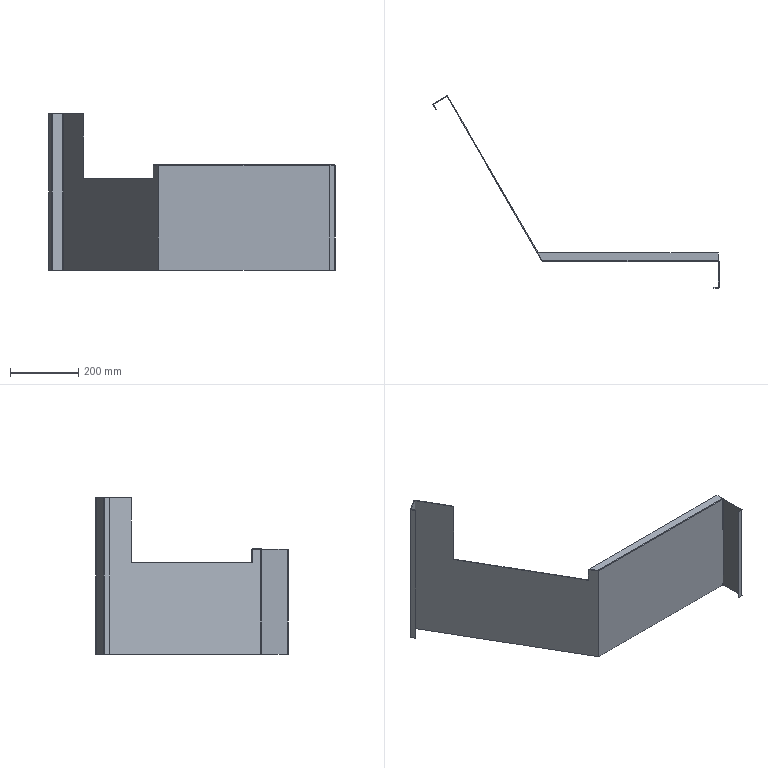Part | STEP file | zh001 | 1 solid | 42 faces | box 840.386 x 564.059 x 459.75 mm | volume 808463 mm3 | plane 28 | cylinder 14 | commonest cylinder face diameters 1 x7 5 x7
STEP:
#1=CARTESIAN_POINT('',(-569.929,497.059,459.75));
#2=VERTEX_POINT('',#1);
#3=CARTESIAN_POINT('',(-569.595,495.809,459.75));
#4=VERTEX_POINT('',#3);
#5=CARTESIAN_POINT('',(-567.429,497.059,459.75));
#6=DIRECTION('',(0.,0.,1.));
#7=DIRECTION('',(-1.,0.,0.));
#8=AXIS2_PLACEMENT_3D('',#5,#6,#7);
#9=CIRCLE('',#8,2.5);
#10=EDGE_CURVE('',#2,#4,#9,.T.);
#11=ORIENTED_EDGE('',*,*,#10,.F.);
#12=CARTESIAN_POINT('',(-569.929,497.059,0.));
#13=VERTEX_POINT('',#12);
#14=CARTESIAN_POINT('',(-569.929,497.059,308.));
#15=DIRECTION('',(0.,0.,-1.));
#16=VECTOR('',#15,1000.);
#17=LINE('',#14,#16);
#18=EDGE_CURVE('',#2,#13,#17,.T.);
#19=ORIENTED_EDGE('',*,*,#18,.T.);
#20=CARTESIAN_POINT('',(-569.595,495.809,0.));
#21=VERTEX_POINT('',#20);
#22=CARTESIAN_POINT('',(-567.429,497.059,0.));
#23=DIRECTION('',(0.,0.,1.));
#24=DIRECTION('',(-1.,0.,0.));
#25=AXIS2_PLACEMENT_3D('',#22,#23,#24);
#26=CIRCLE('',#25,2.5);
#27=EDGE_CURVE('',#13,#21,#26,.T.);
#28=ORIENTED_EDGE('',*,*,#27,.T.);
#29=CARTESIAN_POINT('',(-569.595,495.809,308.));
#30=DIRECTION('',(0.,0.,1.));
#31=VECTOR('',#30,1000.);
#32=LINE('',#29,#31);
#33=EDGE_CURVE('',#21,#4,#32,.T.);
#34=ORIENTED_EDGE('',*,*,#33,.T.);
#35=EDGE_LOOP('',(#11,#19,#28,#34));
#36=FACE_OUTER_BOUND('',#35,.T.);
#37=CARTESIAN_POINT('',(-567.429,497.059,308.));
#38=DIRECTION('',(0.,0.,-1.));
#39=DIRECTION('',(-1.,0.,0.));
#40=AXIS2_PLACEMENT_3D('',#37,#38,#39);
#41=CYLINDRICAL_SURFACE('',#40,2.5);
#42=ADVANCED_FACE('',(#36),#41,.T.);
#43=CARTESIAN_POINT('',(-567.929,497.059,459.75));
#44=VERTEX_POINT('',#43);
#45=CARTESIAN_POINT('',(-567.679,497.492,459.75));
#46=VERTEX_POINT('',#45);
#47=CARTESIAN_POINT('',(-567.429,497.059,459.75));
#48=DIRECTION('',(0.,0.,-1.));
#49=DIRECTION('',(-1.,0.,0.));
#50=AXIS2_PLACEMENT_3D('',#47,#48,#49);
#51=CIRCLE('',#50,0.5);
#52=EDGE_CURVE('',#44,#46,#51,.T.);
#53=ORIENTED_EDGE('',*,*,#52,.F.);
#54=CARTESIAN_POINT('',(-567.929,497.059,0.));
#55=VERTEX_POINT('',#54);
#56=CARTESIAN_POINT('',(-567.929,497.059,308.));
#57=DIRECTION('',(0.,0.,-1.));
#58=VECTOR('',#57,1000.);
#59=LINE('',#56,#58);
#60=EDGE_CURVE('',#44,#55,#59,.T.);
#61=ORIENTED_EDGE('',*,*,#60,.T.);
#62=CARTESIAN_POINT('',(-567.679,497.492,0.));
#63=VERTEX_POINT('',#62);
#64=CARTESIAN_POINT('',(-567.429,497.059,0.));
#65=DIRECTION('',(0.,0.,1.));
#66=DIRECTION('',(-1.,0.,0.));
#67=AXIS2_PLACEMENT_3D('',#64,#65,#66);
#68=CIRCLE('',#67,0.5);
#69=EDGE_CURVE('',#63,#55,#68,.T.);
#70=ORIENTED_EDGE('',*,*,#69,.F.);
#71=CARTESIAN_POINT('',(-567.679,497.492,308.));
#72=DIRECTION('',(0.,0.,-1.));
#73=VECTOR('',#72,1000.);
#74=LINE('',#71,#73);
#75=EDGE_CURVE('',#46,#63,#74,.T.);
#76=ORIENTED_EDGE('',*,*,#75,.F.);
#77=EDGE_LOOP('',(#53,#61,#70,#76));
#78=FACE_OUTER_BOUND('',#77,.T.);
#79=CARTESIAN_POINT('',(-567.429,497.059,308.));
#80=DIRECTION('',(0.,0.,-1.));
#81=DIRECTION('',(-1.,0.,0.));
#82=AXIS2_PLACEMENT_3D('',#79,#80,#81);
#83=CYLINDRICAL_SURFACE('',#82,0.5);
#84=ADVANCED_FACE('',(#78),#83,.F.);
#85=CARTESIAN_POINT('',(-467.543,419.051,459.75));
#86=VERTEX_POINT('',#85);
#87=CARTESIAN_POINT('',(-526.293,520.809,459.75));
#88=VERTEX_POINT('',#87);
#89=CARTESIAN_POINT('',(-247.543,38.,459.75));
#90=DIRECTION('',(-0.5,0.866,0.));
#91=VECTOR('',#90,1000.);
#92=LINE('',#89,#91);
#93=EDGE_CURVE('',#86,#88,#92,.T.);
#94=ORIENTED_EDGE('',*,*,#93,.F.);
#95=CARTESIAN_POINT('',(-467.543,419.051,269.5));
#96=VERTEX_POINT('',#95);
#97=CARTESIAN_POINT('',(-467.543,419.051,308.));
#98=DIRECTION('',(0.,0.,1.));
#99=VECTOR('',#98,1000.);
#100=LINE('',#97,#99);
#101=EDGE_CURVE('',#96,#86,#100,.T.);
#102=ORIENTED_EDGE('',*,*,#101,.F.);
#103=CARTESIAN_POINT('',(-262.471,63.856,269.5));
#104=VERTEX_POINT('',#103);
#105=CARTESIAN_POINT('',(-247.543,38.,269.5));
#106=DIRECTION('',(-0.5,0.866,0.));
#107=VECTOR('',#106,1000.);
#108=LINE('',#105,#107);
#109=EDGE_CURVE('',#104,#96,#108,.T.);
#110=ORIENTED_EDGE('',*,*,#109,.F.);
#111=CARTESIAN_POINT('',(-262.471,63.856,308.));
#112=VERTEX_POINT('',#111);
#113=CARTESIAN_POINT('',(-262.471,63.856,308.));
#114=DIRECTION('',(0.,0.,-1.));
#115=VECTOR('',#114,1000.);
#116=LINE('',#113,#115);
#117=EDGE_CURVE('',#112,#104,#116,.T.);
#118=ORIENTED_EDGE('',*,*,#117,.F.);
#119=CARTESIAN_POINT('',(-247.688,38.25,308.));
#120=VERTEX_POINT('',#119);
#121=CARTESIAN_POINT('',(-247.543,38.,308.));
#122=DIRECTION('',(-0.5,0.866,0.));
#123=VECTOR('',#122,1000.);
#124=LINE('',#121,#123);
#125=EDGE_CURVE('',#120,#112,#124,.T.);
#126=ORIENTED_EDGE('',*,*,#125,.F.);
#127=CARTESIAN_POINT('',(-247.688,38.25,0.));
#128=VERTEX_POINT('',#127);
#129=CARTESIAN_POINT('',(-247.688,38.25,308.));
#130=DIRECTION('',(0.,0.,1.));
#131=VECTOR('',#130,1000.);
#132=LINE('',#129,#131);
#133=EDGE_CURVE('',#128,#120,#132,.T.);
#134=ORIENTED_EDGE('',*,*,#133,.F.);
#135=CARTESIAN_POINT('',(-526.293,520.809,0.));
#136=VERTEX_POINT('',#135);
#137=CARTESIAN_POINT('',(-247.543,38.,0.));
#138=DIRECTION('',(0.5,-0.866,0.));
#139=VECTOR('',#138,1000.);
#140=LINE('',#137,#139);
#141=EDGE_CURVE('',#136,#128,#140,.T.);
#142=ORIENTED_EDGE('',*,*,#141,.F.);
#143=CARTESIAN_POINT('',(-526.293,520.809,308.));
#144=DIRECTION('',(0.,0.,-1.));
#145=VECTOR('',#144,1000.);
#146=LINE('',#143,#145);
#147=EDGE_CURVE('',#88,#136,#146,.T.);
#148=ORIENTED_EDGE('',*,*,#147,.F.);
#149=EDGE_LOOP('',(#94,#102,#110,#118,#126,#134,#142,#148));
#150=FACE_OUTER_BOUND('',#149,.T.);
#151=CARTESIAN_POINT('',(-247.543,38.,308.));
#152=DIRECTION('',(-0.866,-0.5,0.));
#153=DIRECTION('',(0.5,-0.866,0.));
#154=AXIS2_PLACEMENT_3D('',#151,#152,#153);
#155=PLANE('',#154);
#156=ADVANCED_FACE('',(#150),#155,.F.);
#157=CARTESIAN_POINT('',(-529.708,521.724,459.75));
#158=VERTEX_POINT('',#157);
#159=CARTESIAN_POINT('',(-528.458,519.559,459.75));
#160=DIRECTION('',(0.,0.,-1.));
#161=DIRECTION('',(-1.,0.,0.));
#162=AXIS2_PLACEMENT_3D('',#159,#160,#161);
#163=CIRCLE('',#162,2.5);
#164=EDGE_CURVE('',#158,#88,#163,.T.);
#165=ORIENTED_EDGE('',*,*,#164,.T.);
#166=ORIENTED_EDGE('',*,*,#147,.T.);
#167=CARTESIAN_POINT('',(-529.708,521.724,0.));
#168=VERTEX_POINT('',#167);
#169=CARTESIAN_POINT('',(-528.458,519.559,0.));
#170=DIRECTION('',(0.,0.,1.));
#171=DIRECTION('',(-1.,0.,0.));
#172=AXIS2_PLACEMENT_3D('',#169,#170,#171);
#173=CIRCLE('',#172,2.5);
#174=EDGE_CURVE('',#136,#168,#173,.T.);
#175=ORIENTED_EDGE('',*,*,#174,.T.);
#176=CARTESIAN_POINT('',(-529.708,521.724,308.));
#177=DIRECTION('',(0.,0.,1.));
#178=VECTOR('',#177,1000.);
#179=LINE('',#176,#178);
#180=EDGE_CURVE('',#168,#158,#179,.T.);
#181=ORIENTED_EDGE('',*,*,#180,.T.);
#182=EDGE_LOOP('',(#165,#166,#175,#181));
#183=FACE_OUTER_BOUND('',#182,.T.);
#184=CARTESIAN_POINT('',(-528.458,519.559,308.));
#185=DIRECTION('',(0.,0.,-1.));
#186=DIRECTION('',(-1.,0.,0.));
#187=AXIS2_PLACEMENT_3D('',#184,#185,#186);
#188=CYLINDRICAL_SURFACE('',#187,2.5);
#189=ADVANCED_FACE('',(#183),#188,.T.);
#190=CARTESIAN_POINT('',(-528.708,519.992,459.75));
#191=VERTEX_POINT('',#190);
#192=CARTESIAN_POINT('',(-528.025,519.809,459.75));
#193=VERTEX_POINT('',#192);
#194=CARTESIAN_POINT('',(-528.458,519.559,459.75));
#195=DIRECTION('',(0.,0.,-1.));
#196=DIRECTION('',(-1.,0.,0.));
#197=AXIS2_PLACEMENT_3D('',#194,#195,#196);
#198=CIRCLE('',#197,0.5);
#199=EDGE_CURVE('',#191,#193,#198,.T.);
#200=ORIENTED_EDGE('',*,*,#199,.T.);
#201=CARTESIAN_POINT('',(-469.275,418.051,459.75));
#202=VERTEX_POINT('',#201);
#203=CARTESIAN_POINT('',(-528.025,519.809,459.75));
#204=DIRECTION('',(0.5,-0.866,0.));
#205=VECTOR('',#204,1000.);
#206=LINE('',#203,#205);
#207=EDGE_CURVE('',#193,#202,#206,.T.);
#208=ORIENTED_EDGE('',*,*,#207,.T.);
#209=CARTESIAN_POINT('',(-469.275,418.051,459.75));
#210=DIRECTION('',(0.866,0.5,0.));
#211=VECTOR('',#210,1000.);
#212=LINE('',#209,#211);
#213=EDGE_CURVE('',#202,#86,#212,.T.);
#214=ORIENTED_EDGE('',*,*,#213,.T.);
#215=ORIENTED_EDGE('',*,*,#93,.T.);
#216=ORIENTED_EDGE('',*,*,#164,.F.);
#217=CARTESIAN_POINT('',(-568.679,499.224,459.75));
#218=VERTEX_POINT('',#217);
#219=CARTESIAN_POINT('',(-529.708,521.724,459.75));
#220=DIRECTION('',(-0.866,-0.5,0.));
#221=VECTOR('',#220,1000.);
#222=LINE('',#219,#221);
#223=EDGE_CURVE('',#158,#218,#222,.T.);
#224=ORIENTED_EDGE('',*,*,#223,.T.);
#225=CARTESIAN_POINT('',(-567.429,497.059,459.75));
#226=DIRECTION('',(0.,0.,1.));
#227=DIRECTION('',(-1.,0.,0.));
#228=AXIS2_PLACEMENT_3D('',#225,#226,#227);
#229=CIRCLE('',#228,2.5);
#230=EDGE_CURVE('',#218,#2,#229,.T.);
#231=ORIENTED_EDGE('',*,*,#230,.T.);
#232=ORIENTED_EDGE('',*,*,#10,.T.);
#233=CARTESIAN_POINT('',(-561.845,482.386,459.75));
#234=VERTEX_POINT('',#233);
#235=CARTESIAN_POINT('',(-569.595,495.809,459.75));
#236=DIRECTION('',(0.5,-0.866,0.));
#237=VECTOR('',#236,1000.);
#238=LINE('',#235,#237);
#239=EDGE_CURVE('',#4,#234,#238,.T.);
#240=ORIENTED_EDGE('',*,*,#239,.T.);
#241=CARTESIAN_POINT('',(-560.113,483.386,459.75));
#242=VERTEX_POINT('',#241);
#243=CARTESIAN_POINT('',(-561.845,482.386,459.75));
#244=DIRECTION('',(0.866,0.5,0.));
#245=VECTOR('',#244,1000.);
#246=LINE('',#243,#245);
#247=EDGE_CURVE('',#234,#242,#246,.T.);
#248=ORIENTED_EDGE('',*,*,#247,.T.);
#249=CARTESIAN_POINT('',(-567.863,496.809,459.75));
#250=VERTEX_POINT('',#249);
#251=CARTESIAN_POINT('',(-560.113,483.386,459.75));
#252=DIRECTION('',(-0.5,0.866,0.));
#253=VECTOR('',#252,1000.);
#254=LINE('',#251,#253);
#255=EDGE_CURVE('',#242,#250,#254,.T.);
#256=ORIENTED_EDGE('',*,*,#255,.T.);
#257=CARTESIAN_POINT('',(-567.429,497.059,459.75));
#258=DIRECTION('',(0.,0.,-1.));
#259=DIRECTION('',(-1.,0.,0.));
#260=AXIS2_PLACEMENT_3D('',#257,#258,#259);
#261=CIRCLE('',#260,0.5);
#262=EDGE_CURVE('',#250,#44,#261,.T.);
#263=ORIENTED_EDGE('',*,*,#262,.T.);
#264=ORIENTED_EDGE('',*,*,#52,.T.);
#265=CARTESIAN_POINT('',(-567.679,497.492,459.75));
#266=DIRECTION('',(0.866,0.5,0.));
#267=VECTOR('',#266,1000.);
#268=LINE('',#265,#267);
#269=EDGE_CURVE('',#46,#191,#268,.T.);
#270=ORIENTED_EDGE('',*,*,#269,.T.);
#271=EDGE_LOOP('',(#200,#208,#214,#215,#216,#224,#231,#232,#240,#248,#256,#263,#264,#270));
#272=FACE_OUTER_BOUND('',#271,.T.);
#273=CARTESIAN_POINT('',(-528.458,519.559,459.75));
#274=DIRECTION('',(0.,0.,1.));
#275=DIRECTION('',(1.,0.,0.));
#276=AXIS2_PLACEMENT_3D('',#273,#274,#275);
#277=PLANE('',#276);
#278=ADVANCED_FACE('',(#272),#277,.T.);
#279=ORIENTED_EDGE('',*,*,#213,.F.);
#280=CARTESIAN_POINT('',(-469.275,418.051,269.5));
#281=VERTEX_POINT('',#280);
#282=CARTESIAN_POINT('',(-469.275,418.051,308.));
#283=DIRECTION('',(0.,0.,1.));
#284=VECTOR('',#283,1000.);
#285=LINE('',#282,#284);
#286=EDGE_CURVE('',#281,#202,#285,.T.);
#287=ORIENTED_EDGE('',*,*,#286,.F.);
#288=CARTESIAN_POINT('',(-469.275,418.051,269.5));
#289=DIRECTION('',(-0.866,-0.5,0.));
#290=VECTOR('',#289,1000.);
#291=LINE('',#288,#290);
#292=EDGE_CURVE('',#96,#281,#291,.T.);
#293=ORIENTED_EDGE('',*,*,#292,.F.);
#294=ORIENTED_EDGE('',*,*,#101,.T.);
#295=EDGE_LOOP('',(#279,#287,#293,#294));
#296=FACE_OUTER_BOUND('',#295,.T.);
#297=CARTESIAN_POINT('',(-469.275,418.051,308.));
#298=DIRECTION('',(-0.5,0.866,0.));
#299=DIRECTION('',(-0.866,-0.5,0.));
#300=AXIS2_PLACEMENT_3D('',#297,#298,#299);
#301=PLANE('',#300);
#302=ADVANCED_FACE('',(#296),#301,.F.);
#303=ORIENTED_EDGE('',*,*,#292,.T.);
#304=CARTESIAN_POINT('',(-264.203,62.856,269.5));
#305=VERTEX_POINT('',#304);
#306=CARTESIAN_POINT('',(-264.203,62.856,269.5));
#307=DIRECTION('',(-0.5,0.866,0.));
#308=VECTOR('',#307,1000.);
#309=LINE('',#306,#308);
#310=EDGE_CURVE('',#305,#281,#309,.T.);
#311=ORIENTED_EDGE('',*,*,#310,.F.);
#312=CARTESIAN_POINT('',(-262.471,63.856,269.5));
#313=DIRECTION('',(-0.866,-0.5,0.));
#314=VECTOR('',#313,1000.);
#315=LINE('',#312,#314);
#316=EDGE_CURVE('',#104,#305,#315,.T.);
#317=ORIENTED_EDGE('',*,*,#316,.F.);
#318=ORIENTED_EDGE('',*,*,#109,.T.);
#319=EDGE_LOOP('',(#303,#311,#317,#318));
#320=FACE_OUTER_BOUND('',#319,.T.);
#321=CARTESIAN_POINT('',(-469.275,418.051,269.5));
#322=DIRECTION('',(0.,0.,-1.));
#323=DIRECTION('',(0.,1.,0.));
#324=AXIS2_PLACEMENT_3D('',#321,#322,#323);
#325=PLANE('',#324);
#326=ADVANCED_FACE('',(#320),#325,.F.);
#327=ORIENTED_EDGE('',*,*,#316,.T.);
#328=CARTESIAN_POINT('',(-264.203,62.856,308.));
#329=VERTEX_POINT('',#328);
#330=CARTESIAN_POINT('',(-264.203,62.856,308.));
#331=DIRECTION('',(0.,0.,-1.));
#332=VECTOR('',#331,1000.);
#333=LINE('',#330,#332);
#334=EDGE_CURVE('',#329,#305,#333,.T.);
#335=ORIENTED_EDGE('',*,*,#334,.F.);
#336=CARTESIAN_POINT('',(-264.203,62.856,308.));
#337=DIRECTION('',(-0.866,-0.5,0.));
#338=VECTOR('',#337,1000.);
#339=LINE('',#336,#338);
#340=EDGE_CURVE('',#112,#329,#339,.T.);
#341=ORIENTED_EDGE('',*,*,#340,.F.);
#342=ORIENTED_EDGE('',*,*,#117,.T.);
#343=EDGE_LOOP('',(#327,#335,#341,#342));
#344=FACE_OUTER_BOUND('',#343,.T.);
#345=CARTESIAN_POINT('',(-264.203,62.856,308.));
#346=DIRECTION('',(0.5,-0.866,0.));
#347=DIRECTION('',(0.866,0.5,0.));
#348=AXIS2_PLACEMENT_3D('',#345,#346,#347);
#349=PLANE('',#348);
#350=ADVANCED_FACE('',(#344),#349,.F.);
#351=CARTESIAN_POINT('',(-249.42,37.25,308.));
#352=VERTEX_POINT('',#351);
#353=CARTESIAN_POINT('',(-264.203,62.856,308.));
#354=DIRECTION('',(0.5,-0.866,0.));
#355=VECTOR('',#354,1000.);
#356=LINE('',#353,#355);
#357=EDGE_CURVE('',#329,#352,#356,.T.);
#358=ORIENTED_EDGE('',*,*,#357,.T.);
#359=CARTESIAN_POINT('',(-247.255,36.,308.));
#360=VERTEX_POINT('',#359);
#361=CARTESIAN_POINT('',(-247.255,38.5,308.));
#362=DIRECTION('',(0.,0.,1.));
#363=DIRECTION('',(-1.,0.,0.));
#364=AXIS2_PLACEMENT_3D('',#361,#362,#363);
#365=CIRCLE('',#364,2.5);
#366=EDGE_CURVE('',#352,#360,#365,.T.);
#367=ORIENTED_EDGE('',*,*,#366,.T.);
#368=CARTESIAN_POINT('',(-247.255,38.,308.));
#369=VERTEX_POINT('',#368);
#370=CARTESIAN_POINT('',(-247.255,38.,308.));
#371=DIRECTION('',(0.,1.,0.));
#372=VECTOR('',#371,1000.);
#373=LINE('',#370,#372);
#374=EDGE_CURVE('',#360,#369,#373,.T.);
#375=ORIENTED_EDGE('',*,*,#374,.T.);
#376=CARTESIAN_POINT('',(-247.255,38.5,308.));
#377=DIRECTION('',(0.,0.,-1.));
#378=DIRECTION('',(-1.,0.,0.));
#379=AXIS2_PLACEMENT_3D('',#376,#377,#378);
#380=CIRCLE('',#379,0.5);
#381=EDGE_CURVE('',#369,#120,#380,.T.);
#382=ORIENTED_EDGE('',*,*,#381,.T.);
#383=ORIENTED_EDGE('',*,*,#125,.T.);
#384=ORIENTED_EDGE('',*,*,#340,.T.);
#385=EDGE_LOOP('',(#358,#367,#375,#382,#383,#384));
#386=FACE_OUTER_BOUND('',#385,.T.);
#387=CARTESIAN_POINT('',(-528.708,519.992,308.));
#388=DIRECTION('',(0.,0.,1.));
#389=DIRECTION('',(1.,0.,0.));
#390=AXIS2_PLACEMENT_3D('',#387,#388,#389);
#391=PLANE('',#390);
#392=ADVANCED_FACE('',(#386),#391,.T.);
#393=ORIENTED_EDGE('',*,*,#133,.T.);
#394=ORIENTED_EDGE('',*,*,#381,.F.);
#395=CARTESIAN_POINT('',(-247.255,38.,0.));
#396=VERTEX_POINT('',#395);
#397=CARTESIAN_POINT('',(-247.255,38.,308.));
#398=DIRECTION('',(0.,0.,1.));
#399=VECTOR('',#398,1000.);
#400=LINE('',#397,#399);
#401=EDGE_CURVE('',#396,#369,#400,.T.);
#402=ORIENTED_EDGE('',*,*,#401,.F.);
#403=CARTESIAN_POINT('',(-247.255,38.5,0.));
#404=DIRECTION('',(0.,0.,1.));
#405=DIRECTION('',(-1.,0.,0.));
#406=AXIS2_PLACEMENT_3D('',#403,#404,#405);
#407=CIRCLE('',#406,0.5);
#408=EDGE_CURVE('',#128,#396,#407,.T.);
#409=ORIENTED_EDGE('',*,*,#408,.F.);
#410=EDGE_LOOP('',(#393,#394,#402,#409));
#411=FACE_OUTER_BOUND('',#410,.T.);
#412=CARTESIAN_POINT('',(-247.255,38.5,308.));
#413=DIRECTION('',(0.,0.,-1.));
#414=DIRECTION('',(-1.,0.,0.));
#415=AXIS2_PLACEMENT_3D('',#412,#413,#414);
#416=CYLINDRICAL_SURFACE('',#415,0.5);
#417=ADVANCED_FACE('',(#411),#416,.F.);
#418=CARTESIAN_POINT('',(-249.42,37.25,0.));
#419=VERTEX_POINT('',#418);
#420=CARTESIAN_POINT('',(-528.025,519.809,0.));
#421=VERTEX_POINT('',#420);
#422=CARTESIAN_POINT('',(-249.42,37.25,0.));
#423=DIRECTION('',(-0.5,0.866,0.));
#424=VECTOR('',#423,1000.);
#425=LINE('',#422,#424);
#426=EDGE_CURVE('',#419,#421,#425,.T.);
#427=ORIENTED_EDGE('',*,*,#426,.T.);
#428=CARTESIAN_POINT('',(-528.708,519.992,0.));
#429=VERTEX_POINT('',#428);
#430=CARTESIAN_POINT('',(-528.458,519.559,0.));
#431=DIRECTION('',(0.,0.,1.));
#432=DIRECTION('',(-1.,0.,0.));
#433=AXIS2_PLACEMENT_3D('',#430,#431,#432);
#434=CIRCLE('',#433,0.5);
#435=EDGE_CURVE('',#421,#429,#434,.T.);
#436=ORIENTED_EDGE('',*,*,#435,.T.);
#437=CARTESIAN_POINT('',(-526.543,521.242,0.));
#438=DIRECTION('',(0.866,0.5,0.));
#439=VECTOR('',#438,1000.);
#440=LINE('',#437,#439);
#441=EDGE_CURVE('',#63,#429,#440,.T.);
#442=ORIENTED_EDGE('',*,*,#441,.F.);
#443=ORIENTED_EDGE('',*,*,#69,.T.);
#444=CARTESIAN_POINT('',(-567.863,496.809,0.));
#445=VERTEX_POINT('',#444);
#446=CARTESIAN_POINT('',(-567.429,497.059,0.));
#447=DIRECTION('',(0.,0.,1.));
#448=DIRECTION('',(-1.,0.,0.));
#449=AXIS2_PLACEMENT_3D('',#446,#447,#448);
#450=CIRCLE('',#449,0.5);
#451=EDGE_CURVE('',#55,#445,#450,.T.);
#452=ORIENTED_EDGE('',*,*,#451,.T.);
#453=CARTESIAN_POINT('',(-560.113,483.386,0.));
#454=VERTEX_POINT('',#453);
#455=CARTESIAN_POINT('',(-569.113,498.974,0.));
#456=DIRECTION('',(-0.5,0.866,0.));
#457=VECTOR('',#456,1000.);
#458=LINE('',#455,#457);
#459=EDGE_CURVE('',#454,#445,#458,.T.);
#460=ORIENTED_EDGE('',*,*,#459,.F.);
#461=CARTESIAN_POINT('',(-561.845,482.386,0.));
#462=VERTEX_POINT('',#461);
#463=CARTESIAN_POINT('',(-560.113,483.386,0.));
#464=DIRECTION('',(0.866,0.5,0.));
#465=VECTOR('',#464,1000.);
#466=LINE('',#463,#465);
#467=EDGE_CURVE('',#462,#454,#466,.T.);
#468=ORIENTED_EDGE('',*,*,#467,.F.);
#469=CARTESIAN_POINT('',(-570.845,497.974,0.));
#470=DIRECTION('',(-0.5,0.866,0.));
#471=VECTOR('',#470,1000.);
#472=LINE('',#469,#471);
#473=EDGE_CURVE('',#462,#21,#472,.T.);
#474=ORIENTED_EDGE('',*,*,#473,.T.);
#475=ORIENTED_EDGE('',*,*,#27,.F.);
#476=CARTESIAN_POINT('',(-568.679,499.224,0.));
#477=VERTEX_POINT('',#476);
#478=CARTESIAN_POINT('',(-567.429,497.059,0.));
#479=DIRECTION('',(0.,0.,1.));
#480=DIRECTION('',(-1.,0.,0.));
#481=AXIS2_PLACEMENT_3D('',#478,#479,#480);
#482=CIRCLE('',#481,2.5);
#483=EDGE_CURVE('',#477,#13,#482,.T.);
#484=ORIENTED_EDGE('',*,*,#483,.F.);
#485=CARTESIAN_POINT('',(-527.543,522.974,0.));
#486=DIRECTION('',(0.866,0.5,0.));
#487=VECTOR('',#486,1000.);
#488=LINE('',#485,#487);
#489=EDGE_CURVE('',#477,#168,#488,.T.);
#490=ORIENTED_EDGE('',*,*,#489,.T.);
#491=ORIENTED_EDGE('',*,*,#174,.F.);
#492=ORIENTED_EDGE('',*,*,#141,.T.);
#493=ORIENTED_EDGE('',*,*,#408,.T.);
#494=CARTESIAN_POINT('',(267.957,38.,0.));
#495=VERTEX_POINT('',#494);
#496=CARTESIAN_POINT('',(270.457,38.,0.));
#497=DIRECTION('',(1.,0.,0.));
#498=VECTOR('',#497,1000.);
#499=LINE('',#496,#498);
#500=EDGE_CURVE('',#396,#495,#499,.T.);
#501=ORIENTED_EDGE('',*,*,#500,.T.);
#502=CARTESIAN_POINT('',(270.457,35.5,0.));
#503=VERTEX_POINT('',#502);
#504=CARTESIAN_POINT('',(267.957,35.5,0.));
#505=DIRECTION('',(0.,0.,1.));
#506=DIRECTION('',(-1.,0.,0.));
#507=AXIS2_PLACEMENT_3D('',#504,#505,#506);
#508=CIRCLE('',#507,2.5);
#509=EDGE_CURVE('',#503,#495,#508,.T.);
#510=ORIENTED_EDGE('',*,*,#509,.F.);
#511=CARTESIAN_POINT('',(270.457,-39.5,0.));
#512=VERTEX_POINT('',#511);
#513=CARTESIAN_POINT('',(270.457,-42.,0.));
#514=DIRECTION('',(0.,-1.,0.));
#515=VECTOR('',#514,1000.);
#516=LINE('',#513,#515);
#517=EDGE_CURVE('',#503,#512,#516,.T.);
#518=ORIENTED_EDGE('',*,*,#517,.T.);
#519=CARTESIAN_POINT('',(267.957,-42.,0.));
#520=VERTEX_POINT('',#519);
#521=CARTESIAN_POINT('',(267.957,-39.5,0.));
#522=DIRECTION('',(0.,0.,1.));
#523=DIRECTION('',(-1.,0.,0.));
#524=AXIS2_PLACEMENT_3D('',#521,#522,#523);
#525=CIRCLE('',#524,2.5);
#526=EDGE_CURVE('',#520,#512,#525,.T.);
#527=ORIENTED_EDGE('',*,*,#526,.F.);
#528=CARTESIAN_POINT('',(255.457,-42.,0.));
#529=VERTEX_POINT('',#528);
#530=CARTESIAN_POINT('',(270.457,-42.,0.));
#531=DIRECTION('',(-1.,0.,0.));
#532=VECTOR('',#531,1000.);
#533=LINE('',#530,#532);
#534=EDGE_CURVE('',#520,#529,#533,.T.);
#535=ORIENTED_EDGE('',*,*,#534,.T.);
#536=CARTESIAN_POINT('',(255.457,-40.,0.));
#537=VERTEX_POINT('',#536);
#538=CARTESIAN_POINT('',(255.457,497.059,0.));
#539=DIRECTION('',(0.,-1.,0.));
#540=VECTOR('',#539,1000.);
#541=LINE('',#538,#540);
#542=EDGE_CURVE('',#537,#529,#541,.T.);
#543=ORIENTED_EDGE('',*,*,#542,.F.);
#544=CARTESIAN_POINT('',(267.957,-40.,0.));
#545=VERTEX_POINT('',#544);
#546=CARTESIAN_POINT('',(-567.429,-40.,0.));
#547=DIRECTION('',(-1.,0.,0.));
#548=VECTOR('',#547,1000.);
#549=LINE('',#546,#548);
#550=EDGE_CURVE('',#545,#537,#549,.T.);
#551=ORIENTED_EDGE('',*,*,#550,.F.);
#552=CARTESIAN_POINT('',(268.457,-39.5,0.));
#553=VERTEX_POINT('',#552);
#554=CARTESIAN_POINT('',(267.957,-39.5,0.));
#555=DIRECTION('',(0.,0.,1.));
#556=DIRECTION('',(-1.,0.,0.));
#557=AXIS2_PLACEMENT_3D('',#554,#555,#556);
#558=CIRCLE('',#557,0.5);
#559=EDGE_CURVE('',#545,#553,#558,.T.);
#560=ORIENTED_EDGE('',*,*,#559,.T.);
#561=CARTESIAN_POINT('',(268.457,35.5,0.));
#562=VERTEX_POINT('',#561);
#563=CARTESIAN_POINT('',(268.457,-40.,0.));
#564=DIRECTION('',(0.,1.,0.));
#565=VECTOR('',#564,1000.);
#566=LINE('',#563,#565);
#567=EDGE_CURVE('',#553,#562,#566,.T.);
#568=ORIENTED_EDGE('',*,*,#567,.T.);
#569=CARTESIAN_POINT('',(267.957,36.,0.));
#570=VERTEX_POINT('',#569);
#571=CARTESIAN_POINT('',(267.957,35.5,0.));
#572=DIRECTION('',(0.,0.,1.));
#573=DIRECTION('',(-1.,0.,0.));
#574=AXIS2_PLACEMENT_3D('',#571,#572,#573);
#575=CIRCLE('',#574,0.5);
#576=EDGE_CURVE('',#562,#570,#575,.T.);
#577=ORIENTED_EDGE('',*,*,#576,.T.);
#578=CARTESIAN_POINT('',(-247.255,36.,0.));
#579=VERTEX_POINT('',#578);
#580=CARTESIAN_POINT('',(268.457,36.,0.));
#581=DIRECTION('',(-1.,0.,0.));
#582=VECTOR('',#581,1000.);
#583=LINE('',#580,#582);
#584=EDGE_CURVE('',#570,#579,#583,.T.);
#585=ORIENTED_EDGE('',*,*,#584,.T.);
#586=CARTESIAN_POINT('',(-247.255,38.5,0.));
#587=DIRECTION('',(0.,0.,-1.));
#588=DIRECTION('',(-1.,0.,0.));
#589=AXIS2_PLACEMENT_3D('',#586,#587,#588);
#590=CIRCLE('',#589,2.5);
#591=EDGE_CURVE('',#579,#419,#590,.T.);
#592=ORIENTED_EDGE('',*,*,#591,.T.);
#593=EDGE_LOOP('',(#427,#436,#442,#443,#452,#460,#468,#474,#475,#484,#490,#491,#492,#493,#501,#510,#518,#527,#535,#543,#551,#560,#568,#577,#585,#592));
#594=FACE_OUTER_BOUND('',#593,.T.);
#595=CARTESIAN_POINT('',(-247.255,36.,0.));
#596=DIRECTION('',(0.,0.,-1.));
#597=DIRECTION('',(-1.,0.,0.));
#598=AXIS2_PLACEMENT_3D('',#595,#596,#597);
#599=PLANE('',#598);
#600=ADVANCED_FACE('',(#594),#599,.T.);
#601=CARTESIAN_POINT('',(-568.679,499.224,308.));
#602=DIRECTION('',(0.,0.,-1.));
#603=VECTOR('',#602,1000.);
#604=LINE('',#601,#603);
#605=EDGE_CURVE('',#218,#477,#604,.T.);
#606=ORIENTED_EDGE('',*,*,#605,.F.);
#607=ORIENTED_EDGE('',*,*,#223,.F.);
#608=ORIENTED_EDGE('',*,*,#180,.F.);
#609=ORIENTED_EDGE('',*,*,#489,.F.);
#610=EDGE_LOOP('',(#606,#607,#608,#609));
#611=FACE_OUTER_BOUND('',#610,.T.);
#612=CARTESIAN_POINT('',(-527.543,522.974,308.));
#613=DIRECTION('',(0.5,-0.866,0.));
#614=DIRECTION('',(0.866,0.5,0.));
#615=AXIS2_PLACEMENT_3D('',#612,#613,#614);
#616=PLANE('',#615);
#617=ADVANCED_FACE('',(#611),#616,.F.);
#618=ORIENTED_EDGE('',*,*,#334,.T.);
#619=ORIENTED_EDGE('',*,*,#310,.T.);
#620=ORIENTED_EDGE('',*,*,#286,.T.);
#621=ORIENTED_EDGE('',*,*,#207,.F.);
#622=CARTESIAN_POINT('',(-528.025,519.809,308.));
#623=DIRECTION('',(0.,0.,-1.));
#624=VECTOR('',#623,1000.);
#625=LINE('',#622,#624);
#626=EDGE_CURVE('',#193,#421,#625,.T.);
#627=ORIENTED_EDGE('',*,*,#626,.T.);
#628=ORIENTED_EDGE('',*,*,#426,.F.);
#629=CARTESIAN_POINT('',(-249.42,37.25,308.));
#630=DIRECTION('',(0.,0.,1.));
#631=VECTOR('',#630,1000.);
#632=LINE('',#629,#631);
#633=EDGE_CURVE('',#419,#352,#632,.T.);
#634=ORIENTED_EDGE('',*,*,#633,.T.);
#635=ORIENTED_EDGE('',*,*,#357,.F.);
#636=EDGE_LOOP('',(#618,#619,#620,#621,#627,#628,#634,#635));
#637=FACE_OUTER_BOUND('',#636,.T.);
#638=CARTESIAN_POINT('',(-249.275,37.,308.));
#639=DIRECTION('',(-0.866,-0.5,0.));
#640=DIRECTION('',(0.5,-0.866,0.));
#641=AXIS2_PLACEMENT_3D('',#638,#639,#640);
#642=PLANE('',#641);
#643=ADVANCED_FACE('',(#637),#642,.T.);
#644=ORIENTED_EDGE('',*,*,#269,.F.);
#645=ORIENTED_EDGE('',*,*,#75,.T.);
#646=ORIENTED_EDGE('',*,*,#441,.T.);
#647=CARTESIAN_POINT('',(-528.708,519.992,308.));
#648=DIRECTION('',(0.,0.,1.));
#649=VECTOR('',#648,1000.);
#650=LINE('',#647,#649);
#651=EDGE_CURVE('',#429,#191,#650,.T.);
#652=ORIENTED_EDGE('',*,*,#651,.T.);
#653=EDGE_LOOP('',(#644,#645,#646,#652));
#654=FACE_OUTER_BOUND('',#653,.T.);
#655=CARTESIAN_POINT('',(-526.543,521.242,308.));
#656=DIRECTION('',(0.5,-0.866,0.));
#657=DIRECTION('',(0.866,0.5,0.));
#658=AXIS2_PLACEMENT_3D('',#655,#656,#657);
#659=PLANE('',#658);
#660=ADVANCED_FACE('',(#654),#659,.T.);
#661=ORIENTED_EDGE('',*,*,#255,.F.);
#662=CARTESIAN_POINT('',(-560.113,483.386,308.));
#663=DIRECTION('',(0.,0.,-1.));
#664=VECTOR('',#663,1000.);
#665=LINE('',#662,#664);
#666=EDGE_CURVE('',#242,#454,#665,.T.);
#667=ORIENTED_EDGE('',*,*,#666,.T.);
#668=ORIENTED_EDGE('',*,*,#459,.T.);
#669=CARTESIAN_POINT('',(-567.863,496.809,308.));
#670=DIRECTION('',(0.,0.,1.));
#671=VECTOR('',#670,1000.);
#672=LINE('',#669,#671);
#673=EDGE_CURVE('',#445,#250,#672,.T.);
#674=ORIENTED_EDGE('',*,*,#673,.T.);
#675=EDGE_LOOP('',(#661,#667,#668,#674));
#676=FACE_OUTER_BOUND('',#675,.T.);
#677=CARTESIAN_POINT('',(-569.113,498.974,308.));
#678=DIRECTION('',(0.866,0.5,0.));
#679=DIRECTION('',(-0.5,0.866,0.));
#680=AXIS2_PLACEMENT_3D('',#677,#678,#679);
#681=PLANE('',#680);
#682=ADVANCED_FACE('',(#676),#681,.T.);
#683=ORIENTED_EDGE('',*,*,#247,.F.);
#684=CARTESIAN_POINT('',(-561.845,482.386,308.));
#685=DIRECTION('',(0.,0.,-1.));
#686=VECTOR('',#685,1000.);
#687=LINE('',#684,#686);
#688=EDGE_CURVE('',#234,#462,#687,.T.);
#689=ORIENTED_EDGE('',*,*,#688,.T.);
#690=ORIENTED_EDGE('',*,*,#467,.T.);
#691=ORIENTED_EDGE('',*,*,#666,.F.);
#692=EDGE_LOOP('',(#683,#689,#690,#691));
#693=FACE_OUTER_BOUND('',#692,.T.);
#694=CARTESIAN_POINT('',(-560.113,483.386,308.));
#695=DIRECTION('',(0.5,-0.866,0.));
#696=DIRECTION('',(0.866,0.5,0.));
#697=AXIS2_PLACEMENT_3D('',#694,#695,#696);
#698=PLANE('',#697);
#699=ADVANCED_FACE('',(#693),#698,.T.);
#700=ORIENTED_EDGE('',*,*,#688,.F.);
#701=ORIENTED_EDGE('',*,*,#239,.F.);
#702=ORIENTED_EDGE('',*,*,#33,.F.);
#703=ORIENTED_EDGE('',*,*,#473,.F.);
#704=EDGE_LOOP('',(#700,#701,#702,#703));
#705=FACE_OUTER_BOUND('',#704,.T.);
#706=CARTESIAN_POINT('',(-570.845,497.974,308.));
#707=DIRECTION('',(0.866,0.5,0.));
#708=DIRECTION('',(-0.5,0.866,0.));
#709=AXIS2_PLACEMENT_3D('',#706,#707,#708);
#710=PLANE('',#709);
#711=ADVANCED_FACE('',(#705),#710,.F.);
#712=ORIENTED_EDGE('',*,*,#18,.F.);
#713=ORIENTED_EDGE('',*,*,#230,.F.);
#714=ORIENTED_EDGE('',*,*,#605,.T.);
#715=ORIENTED_EDGE('',*,*,#483,.T.);
#716=EDGE_LOOP('',(#712,#713,#714,#715));
#717=FACE_OUTER_BOUND('',#716,.T.);
#718=CARTESIAN_POINT('',(-567.429,497.059,308.));
#719=DIRECTION('',(0.,0.,-1.));
#720=DIRECTION('',(-1.,0.,0.));
#721=AXIS2_PLACEMENT_3D('',#718,#719,#720);
#722=CYLINDRICAL_SURFACE('',#721,2.5);
#723=ADVANCED_FACE('',(#717),#722,.T.);
#724=ORIENTED_EDGE('',*,*,#401,.T.);
#725=CARTESIAN_POINT('',(267.957,38.,308.));
#726=VERTEX_POINT('',#725);
#727=CARTESIAN_POINT('',(270.457,38.,308.));
#728=DIRECTION('',(-1.,0.,0.));
#729=VECTOR('',#728,1000.);
#730=LINE('',#727,#729);
#731=EDGE_CURVE('',#726,#369,#730,.T.);
#732=ORIENTED_EDGE('',*,*,#731,.F.);
#733=CARTESIAN_POINT('',(267.957,38.,308.));
#734=DIRECTION('',(0.,0.,1.));
#735=VECTOR('',#734,1000.);
#736=LINE('',#733,#735);
#737=EDGE_CURVE('',#495,#726,#736,.T.);
#738=ORIENTED_EDGE('',*,*,#737,.F.);
#739=ORIENTED_EDGE('',*,*,#500,.F.);
#740=EDGE_LOOP('',(#724,#732,#738,#739));
#741=FACE_OUTER_BOUND('',#740,.T.);
#742=CARTESIAN_POINT('',(270.457,38.,308.));
#743=DIRECTION('',(0.,-1.,0.));
#744=DIRECTION('',(1.,0.,0.));
#745=AXIS2_PLACEMENT_3D('',#742,#743,#744);
#746=PLANE('',#745);
#747=ADVANCED_FACE('',(#741),#746,.F.);
#748=ORIENTED_EDGE('',*,*,#366,.F.);
#749=ORIENTED_EDGE('',*,*,#633,.F.);
#750=ORIENTED_EDGE('',*,*,#591,.F.);
#751=CARTESIAN_POINT('',(-247.255,36.,308.));
#752=DIRECTION('',(0.,0.,1.));
#753=VECTOR('',#752,1000.);
#754=LINE('',#751,#753);
#755=EDGE_CURVE('',#579,#360,#754,.T.);
#756=ORIENTED_EDGE('',*,*,#755,.T.);
#757=EDGE_LOOP('',(#748,#749,#750,#756));
#758=FACE_OUTER_BOUND('',#757,.T.);
#759=CARTESIAN_POINT('',(-247.255,38.5,308.));
#760=DIRECTION('',(0.,0.,-1.));
#761=DIRECTION('',(-1.,0.,0.));
#762=AXIS2_PLACEMENT_3D('',#759,#760,#761);
#763=CYLINDRICAL_SURFACE('',#762,2.5);
#764=ADVANCED_FACE('',(#758),#763,.T.);
#765=ORIENTED_EDGE('',*,*,#626,.F.);
#766=ORIENTED_EDGE('',*,*,#199,.F.);
#767=ORIENTED_EDGE('',*,*,#651,.F.);
#768=ORIENTED_EDGE('',*,*,#435,.F.);
#769=EDGE_LOOP('',(#765,#766,#767,#768));
#770=FACE_OUTER_BOUND('',#769,.T.);
#771=CARTESIAN_POINT('',(-528.458,519.559,308.));
#772=DIRECTION('',(0.,0.,-1.));
#773=DIRECTION('',(-1.,0.,0.));
#774=AXIS2_PLACEMENT_3D('',#771,#772,#773);
#775=CYLINDRICAL_SURFACE('',#774,0.5);
#776=ADVANCED_FACE('',(#770),#775,.F.);
#777=ORIENTED_EDGE('',*,*,#60,.F.);
#778=ORIENTED_EDGE('',*,*,#262,.F.);
#779=ORIENTED_EDGE('',*,*,#673,.F.);
#780=ORIENTED_EDGE('',*,*,#451,.F.);
#781=EDGE_LOOP('',(#777,#778,#779,#780));
#782=FACE_OUTER_BOUND('',#781,.T.);
#783=CARTESIAN_POINT('',(-567.429,497.059,308.));
#784=DIRECTION('',(0.,0.,-1.));
#785=DIRECTION('',(-1.,0.,0.));
#786=AXIS2_PLACEMENT_3D('',#783,#784,#785);
#787=CYLINDRICAL_SURFACE('',#786,0.5);
#788=ADVANCED_FACE('',(#782),#787,.F.);
#789=ORIENTED_EDGE('',*,*,#374,.F.);
#790=CARTESIAN_POINT('',(-247.255,38.5,310.5));
#791=VERTEX_POINT('',#790);
#792=CARTESIAN_POINT('',(-247.255,38.5,308.));
#793=DIRECTION('',(-1.,0.,0.));
#794=DIRECTION('',(0.,0.,-1.));
#795=AXIS2_PLACEMENT_3D('',#792,#793,#794);
#796=CIRCLE('',#795,2.5);
#797=EDGE_CURVE('',#360,#791,#796,.T.);
#798=ORIENTED_EDGE('',*,*,#797,.T.);
#799=CARTESIAN_POINT('',(-247.255,38.6,310.5));
#800=VERTEX_POINT('',#799);
#801=CARTESIAN_POINT('',(-247.255,38.,310.5));
#802=DIRECTION('',(0.,-1.,0.));
#803=VECTOR('',#802,1000.);
#804=LINE('',#801,#803);
#805=EDGE_CURVE('',#800,#791,#804,.T.);
#806=ORIENTED_EDGE('',*,*,#805,.F.);
#807=CARTESIAN_POINT('',(-247.255,38.6,308.5));
#808=VERTEX_POINT('',#807);
#809=CARTESIAN_POINT('',(-247.255,38.6,310.5));
#810=DIRECTION('',(0.,0.,1.));
#811=VECTOR('',#810,1000.);
#812=LINE('',#809,#811);
#813=EDGE_CURVE('',#808,#800,#812,.T.);
#814=ORIENTED_EDGE('',*,*,#813,.F.);
#815=CARTESIAN_POINT('',(-247.255,38.5,308.5));
#816=VERTEX_POINT('',#815);
#817=CARTESIAN_POINT('',(-247.255,38.,308.5));
#818=DIRECTION('',(0.,1.,0.));
#819=VECTOR('',#818,1000.);
#820=LINE('',#817,#819);
#821=EDGE_CURVE('',#816,#808,#820,.T.);
#822=ORIENTED_EDGE('',*,*,#821,.F.);
#823=CARTESIAN_POINT('',(-247.255,38.5,308.));
#824=DIRECTION('',(1.,0.,0.));
#825=DIRECTION('',(0.,0.,-1.));
#826=AXIS2_PLACEMENT_3D('',#823,#824,#825);
#827=CIRCLE('',#826,0.5);
#828=EDGE_CURVE('',#816,#369,#827,.T.);
#829=ORIENTED_EDGE('',*,*,#828,.T.);
#830=EDGE_LOOP('',(#789,#798,#806,#814,#822,#829));
#831=FACE_OUTER_BOUND('',#830,.T.);
#832=CARTESIAN_POINT('',(-247.255,38.5,308.));
#833=DIRECTION('',(-1.,0.,0.));
#834=DIRECTION('',(0.,0.,1.));
#835=AXIS2_PLACEMENT_3D('',#832,#833,#834);
#836=PLANE('',#835);
#837=ADVANCED_FACE('',(#831),#836,.T.);
#838=ORIENTED_EDGE('',*,*,#828,.F.);
#839=CARTESIAN_POINT('',(267.957,38.5,308.5));
#840=VERTEX_POINT('',#839);
#841=CARTESIAN_POINT('',(267.957,38.5,308.5));
#842=DIRECTION('',(-1.,0.,0.));
#843=VECTOR('',#842,1000.);
#844=LINE('',#841,#843);
#845=EDGE_CURVE('',#840,#816,#844,.T.);
#846=ORIENTED_EDGE('',*,*,#845,.F.);
#847=CARTESIAN_POINT('',(267.957,38.5,308.));
#848=DIRECTION('',(1.,0.,0.));
#849=DIRECTION('',(0.,0.,-1.));
#850=AXIS2_PLACEMENT_3D('',#847,#848,#849);
#851=CIRCLE('',#850,0.5);
#852=EDGE_CURVE('',#840,#726,#851,.T.);
#853=ORIENTED_EDGE('',*,*,#852,.T.);
#854=ORIENTED_EDGE('',*,*,#731,.T.);
#855=EDGE_LOOP('',(#838,#846,#853,#854));
#856=FACE_OUTER_BOUND('',#855,.T.);
#857=CARTESIAN_POINT('',(267.957,38.5,308.));
#858=DIRECTION('',(1.,0.,0.));
#859=DIRECTION('',(0.,0.,-1.));
#860=AXIS2_PLACEMENT_3D('',#857,#858,#859);
#861=CYLINDRICAL_SURFACE('',#860,0.5);
#862=ADVANCED_FACE('',(#856),#861,.F.);
#863=CARTESIAN_POINT('',(270.457,35.5,308.));
#864=VERTEX_POINT('',#863);
#865=CARTESIAN_POINT('',(267.957,35.5,308.));
#866=DIRECTION('',(0.,0.,-1.));
#867=DIRECTION('',(-1.,0.,0.));
#868=AXIS2_PLACEMENT_3D('',#865,#866,#867);
#869=CIRCLE('',#868,2.5);
#870=EDGE_CURVE('',#726,#864,#869,.T.);
#871=ORIENTED_EDGE('',*,*,#870,.T.);
#872=CARTESIAN_POINT('',(270.457,35.5,308.));
#873=DIRECTION('',(0.,0.,-1.));
#874=VECTOR('',#873,1000.);
#875=LINE('',#872,#874);
#876=EDGE_CURVE('',#864,#503,#875,.T.);
#877=ORIENTED_EDGE('',*,*,#876,.T.);
#878=ORIENTED_EDGE('',*,*,#509,.T.);
#879=ORIENTED_EDGE('',*,*,#737,.T.);
#880=EDGE_LOOP('',(#871,#877,#878,#879));
#881=FACE_OUTER_BOUND('',#880,.T.);
#882=CARTESIAN_POINT('',(267.957,35.5,308.));
#883=DIRECTION('',(0.,0.,-1.));
#884=DIRECTION('',(-1.,0.,0.));
#885=AXIS2_PLACEMENT_3D('',#882,#883,#884);
#886=CYLINDRICAL_SURFACE('',#885,2.5);
#887=ADVANCED_FACE('',(#881),#886,.T.);
#888=CARTESIAN_POINT('',(267.957,36.,308.));
#889=VERTEX_POINT('',#888);
#890=CARTESIAN_POINT('',(270.457,36.,308.));
#891=DIRECTION('',(-1.,0.,0.));
#892=VECTOR('',#891,1000.);
#893=LINE('',#890,#892);
#894=EDGE_CURVE('',#889,#360,#893,.T.);
#895=ORIENTED_EDGE('',*,*,#894,.T.);
#896=ORIENTED_EDGE('',*,*,#755,.F.);
#897=ORIENTED_EDGE('',*,*,#584,.F.);
#898=CARTESIAN_POINT('',(267.957,36.,308.));
#899=DIRECTION('',(0.,0.,1.));
#900=VECTOR('',#899,1000.);
#901=LINE('',#898,#900);
#902=EDGE_CURVE('',#570,#889,#901,.T.);
#903=ORIENTED_EDGE('',*,*,#902,.T.);
#904=EDGE_LOOP('',(#895,#896,#897,#903));
#905=FACE_OUTER_BOUND('',#904,.T.);
#906=CARTESIAN_POINT('',(270.457,36.,308.));
#907=DIRECTION('',(0.,-1.,0.));
#908=DIRECTION('',(1.,0.,0.));
#909=AXIS2_PLACEMENT_3D('',#906,#907,#908);
#910=PLANE('',#909);
#911=ADVANCED_FACE('',(#905),#910,.T.);
#912=CARTESIAN_POINT('',(267.957,38.5,310.5));
#913=VERTEX_POINT('',#912);
#914=CARTESIAN_POINT('',(267.957,38.5,310.5));
#915=DIRECTION('',(-1.,0.,0.));
#916=VECTOR('',#915,1000.);
#917=LINE('',#914,#916);
#918=EDGE_CURVE('',#913,#791,#917,.T.);
#919=ORIENTED_EDGE('',*,*,#918,.T.);
#920=ORIENTED_EDGE('',*,*,#797,.F.);
#921=ORIENTED_EDGE('',*,*,#894,.F.);
#922=CARTESIAN_POINT('',(267.957,38.5,308.));
#923=DIRECTION('',(-1.,0.,0.));
#924=DIRECTION('',(0.,0.,-1.));
#925=AXIS2_PLACEMENT_3D('',#922,#923,#924);
#926=CIRCLE('',#925,2.5);
#927=EDGE_CURVE('',#889,#913,#926,.T.);
#928=ORIENTED_EDGE('',*,*,#927,.T.);
#929=EDGE_LOOP('',(#919,#920,#921,#928));
#930=FACE_OUTER_BOUND('',#929,.T.);
#931=CARTESIAN_POINT('',(267.957,38.5,308.));
#932=DIRECTION('',(1.,0.,0.));
#933=DIRECTION('',(0.,0.,-1.));
#934=AXIS2_PLACEMENT_3D('',#931,#932,#933);
#935=CYLINDRICAL_SURFACE('',#934,2.5);
#936=ADVANCED_FACE('',(#930),#935,.T.);
#937=CARTESIAN_POINT('',(-249.463,37.325,308.5));
#938=VERTEX_POINT('',#937);
#939=CARTESIAN_POINT('',(-263.132,61.,308.5));
#940=VERTEX_POINT('',#939);
#941=CARTESIAN_POINT('',(-249.463,37.325,308.5));
#942=DIRECTION('',(-0.5,0.866,0.));
#943=VECTOR('',#942,1000.);
#944=LINE('',#941,#943);
#945=EDGE_CURVE('',#938,#940,#944,.T.);
#946=ORIENTED_EDGE('',*,*,#945,.T.);
#947=CARTESIAN_POINT('',(267.957,61.,308.5));
#948=VERTEX_POINT('',#947);
#949=CARTESIAN_POINT('',(0.,61.,308.5));
#950=DIRECTION('',(1.,0.,0.));
#951=VECTOR('',#950,1000.);
#952=LINE('',#949,#951);
#953=EDGE_CURVE('',#940,#948,#952,.T.);
#954=ORIENTED_EDGE('',*,*,#953,.T.);
#955=CARTESIAN_POINT('',(267.957,0.,308.5));
#956=DIRECTION('',(0.,-1.,0.));
#957=VECTOR('',#956,1000.);
#958=LINE('',#955,#957);
#959=EDGE_CURVE('',#948,#840,#958,.T.);
#960=ORIENTED_EDGE('',*,*,#959,.T.);
#961=ORIENTED_EDGE('',*,*,#845,.T.);
#962=ORIENTED_EDGE('',*,*,#821,.T.);
#963=CARTESIAN_POINT('',(-247.255,38.6,308.5));
#964=DIRECTION('',(-0.866,-0.5,0.));
#965=VECTOR('',#964,1000.);
#966=LINE('',#963,#965);
#967=EDGE_CURVE('',#808,#938,#966,.T.);
#968=ORIENTED_EDGE('',*,*,#967,.T.);
#969=EDGE_LOOP('',(#946,#954,#960,#961,#962,#968));
#970=FACE_OUTER_BOUND('',#969,.T.);
#971=CARTESIAN_POINT('',(0.,0.,308.5));
#972=DIRECTION('',(0.,0.,-1.));
#973=DIRECTION('',(-1.,0.,0.));
#974=AXIS2_PLACEMENT_3D('',#971,#972,#973);
#975=PLANE('',#974);
#976=ADVANCED_FACE('',(#970),#975,.T.);
#977=ORIENTED_EDGE('',*,*,#876,.F.);
#978=CARTESIAN_POINT('',(270.457,-39.5,308.));
#979=VERTEX_POINT('',#978);
#980=CARTESIAN_POINT('',(270.457,-42.,308.));
#981=DIRECTION('',(0.,1.,0.));
#982=VECTOR('',#981,1000.);
#983=LINE('',#980,#982);
#984=EDGE_CURVE('',#979,#864,#983,.T.);
#985=ORIENTED_EDGE('',*,*,#984,.F.);
#986=CARTESIAN_POINT('',(270.457,-39.5,308.));
#987=DIRECTION('',(0.,0.,1.));
#988=VECTOR('',#987,1000.);
#989=LINE('',#986,#988);
#990=EDGE_CURVE('',#512,#979,#989,.T.);
#991=ORIENTED_EDGE('',*,*,#990,.F.);
#992=ORIENTED_EDGE('',*,*,#517,.F.);
#993=EDGE_LOOP('',(#977,#985,#991,#992));
#994=FACE_OUTER_BOUND('',#993,.T.);
#995=CARTESIAN_POINT('',(270.457,-42.,308.));
#996=DIRECTION('',(-1.,0.,0.));
#997=DIRECTION('',(0.,-1.,0.));
#998=AXIS2_PLACEMENT_3D('',#995,#996,#997);
#999=PLANE('',#998);
#1000=ADVANCED_FACE('',(#994),#999,.F.);
#1001=CARTESIAN_POINT('',(267.957,35.5,308.));
#1002=DIRECTION('',(0.,-1.,0.));
#1003=VECTOR('',#1002,1000.);
#1004=LINE('',#1001,#1003);
#1005=EDGE_CURVE('',#726,#889,#1004,.T.);
#1006=ORIENTED_EDGE('',*,*,#1005,.T.);
#1007=CARTESIAN_POINT('',(268.457,35.5,308.));
#1008=VERTEX_POINT('',#1007);
#1009=CARTESIAN_POINT('',(267.957,35.5,308.));
#1010=DIRECTION('',(0.,0.,-1.));
#1011=DIRECTION('',(-1.,0.,0.));
#1012=AXIS2_PLACEMENT_3D('',#1009,#1010,#1011);
#1013=CIRCLE('',#1012,0.5);
#1014=EDGE_CURVE('',#889,#1008,#1013,.T.);
#1015=ORIENTED_EDGE('',*,*,#1014,.T.);
#1016=CARTESIAN_POINT('',(268.457,-39.5,308.));
#1017=VERTEX_POINT('',#1016);
#1018=CARTESIAN_POINT('',(268.457,36.,308.));
#1019=DIRECTION('',(0.,-1.,0.));
#1020=VECTOR('',#1019,1000.);
#1021=LINE('',#1018,#1020);
#1022=EDGE_CURVE('',#1008,#1017,#1021,.T.);
#1023=ORIENTED_EDGE('',*,*,#1022,.T.);
#1024=CARTESIAN_POINT('',(267.957,-40.,308.));
#1025=VERTEX_POINT('',#1024);
#1026=CARTESIAN_POINT('',(267.957,-39.5,308.));
#1027=DIRECTION('',(0.,0.,-1.));
#1028=DIRECTION('',(-1.,0.,0.));
#1029=AXIS2_PLACEMENT_3D('',#1026,#1027,#1028);
#1030=CIRCLE('',#1029,0.5);
#1031=EDGE_CURVE('',#1017,#1025,#1030,.T.);
#1032=ORIENTED_EDGE('',*,*,#1031,.T.);
#1033=CARTESIAN_POINT('',(255.457,-40.,308.));
#1034=VERTEX_POINT('',#1033);
#1035=CARTESIAN_POINT('',(268.457,-40.,308.));
#1036=DIRECTION('',(-1.,0.,0.));
#1037=VECTOR('',#1036,1000.);
#1038=LINE('',#1035,#1037);
#1039=EDGE_CURVE('',#1025,#1034,#1038,.T.);
#1040=ORIENTED_EDGE('',*,*,#1039,.T.);
#1041=CARTESIAN_POINT('',(255.457,-42.,308.));
#1042=VERTEX_POINT('',#1041);
#1043=CARTESIAN_POINT('',(255.457,-39.5,308.));
#1044=DIRECTION('',(0.,-1.,0.));
#1045=VECTOR('',#1044,1000.);
#1046=LINE('',#1043,#1045);
#1047=EDGE_CURVE('',#1034,#1042,#1046,.T.);
#1048=ORIENTED_EDGE('',*,*,#1047,.T.);
#1049=CARTESIAN_POINT('',(267.957,-42.,308.));
#1050=VERTEX_POINT('',#1049);
#1051=CARTESIAN_POINT('',(270.457,-42.,308.));
#1052=DIRECTION('',(1.,0.,0.));
#1053=VECTOR('',#1052,1000.);
#1054=LINE('',#1051,#1053);
#1055=EDGE_CURVE('',#1042,#1050,#1054,.T.);
#1056=ORIENTED_EDGE('',*,*,#1055,.T.);
#1057=CARTESIAN_POINT('',(267.957,-39.5,308.));
#1058=DIRECTION('',(0.,0.,-1.));
#1059=DIRECTION('',(-1.,0.,0.));
#1060=AXIS2_PLACEMENT_3D('',#1057,#1058,#1059);
#1061=CIRCLE('',#1060,2.5);
#1062=EDGE_CURVE('',#979,#1050,#1061,.T.);
#1063=ORIENTED_EDGE('',*,*,#1062,.F.);
#1064=ORIENTED_EDGE('',*,*,#984,.T.);
#1065=ORIENTED_EDGE('',*,*,#870,.F.);
#1066=EDGE_LOOP('',(#1006,#1015,#1023,#1032,#1040,#1048,#1056,#1063,#1064,#1065));
#1067=FACE_OUTER_BOUND('',#1066,.T.);
#1068=CARTESIAN_POINT('',(270.457,35.5,308.));
#1069=DIRECTION('',(0.,0.,1.));
#1070=DIRECTION('',(1.,0.,0.));
#1071=AXIS2_PLACEMENT_3D('',#1068,#1069,#1070);
#1072=PLANE('',#1071);
#1073=ADVANCED_FACE('',(#1067),#1072,.T.);
#1074=CARTESIAN_POINT('',(268.457,35.5,308.));
#1075=DIRECTION('',(0.,0.,-1.));
#1076=VECTOR('',#1075,1000.);
#1077=LINE('',#1074,#1076);
#1078=EDGE_CURVE('',#1008,#562,#1077,.T.);
#1079=ORIENTED_EDGE('',*,*,#1078,.F.);
#1080=ORIENTED_EDGE('',*,*,#1014,.F.);
#1081=ORIENTED_EDGE('',*,*,#902,.F.);
#1082=ORIENTED_EDGE('',*,*,#576,.F.);
#1083=EDGE_LOOP('',(#1079,#1080,#1081,#1082));
#1084=FACE_OUTER_BOUND('',#1083,.T.);
#1085=CARTESIAN_POINT('',(267.957,35.5,308.));
#1086=DIRECTION('',(0.,0.,-1.));
#1087=DIRECTION('',(-1.,0.,0.));
#1088=AXIS2_PLACEMENT_3D('',#1085,#1086,#1087);
#1089=CYLINDRICAL_SURFACE('',#1088,0.5);
#1090=ADVANCED_FACE('',(#1084),#1089,.F.);
#1091=CARTESIAN_POINT('',(267.957,61.,310.5));
#1092=VERTEX_POINT('',#1091);
#1093=CARTESIAN_POINT('',(267.957,0.,310.5));
#1094=DIRECTION('',(0.,-1.,0.));
#1095=VECTOR('',#1094,1000.);
#1096=LINE('',#1093,#1095);
#1097=EDGE_CURVE('',#1092,#913,#1096,.T.);
#1098=ORIENTED_EDGE('',*,*,#1097,.F.);
#1099=CARTESIAN_POINT('',(-263.132,61.,310.5));
#1100=VERTEX_POINT('',#1099);
#1101=CARTESIAN_POINT('',(0.,61.,310.5));
#1102=DIRECTION('',(1.,0.,0.));
#1103=VECTOR('',#1102,1000.);
#1104=LINE('',#1101,#1103);
#1105=EDGE_CURVE('',#1100,#1092,#1104,.T.);
#1106=ORIENTED_EDGE('',*,*,#1105,.F.);
#1107=CARTESIAN_POINT('',(-249.463,37.325,310.5));
#1108=VERTEX_POINT('',#1107);
#1109=CARTESIAN_POINT('',(-249.463,37.325,310.5));
#1110=DIRECTION('',(-0.5,0.866,0.));
#1111=VECTOR('',#1110,1000.);
#1112=LINE('',#1109,#1111);
#1113=EDGE_CURVE('',#1108,#1100,#1112,.T.);
#1114=ORIENTED_EDGE('',*,*,#1113,.F.);
#1115=CARTESIAN_POINT('',(-247.255,38.6,310.5));
#1116=DIRECTION('',(-0.866,-0.5,0.));
#1117=VECTOR('',#1116,1000.);
#1118=LINE('',#1115,#1117);
#1119=EDGE_CURVE('',#800,#1108,#1118,.T.);
#1120=ORIENTED_EDGE('',*,*,#1119,.F.);
#1121=ORIENTED_EDGE('',*,*,#805,.T.);
#1122=ORIENTED_EDGE('',*,*,#918,.F.);
#1123=EDGE_LOOP('',(#1098,#1106,#1114,#1120,#1121,#1122));
#1124=FACE_OUTER_BOUND('',#1123,.T.);
#1125=CARTESIAN_POINT('',(0.,0.,310.5));
#1126=DIRECTION('',(0.,0.,-1.));
#1127=DIRECTION('',(-1.,0.,0.));
#1128=AXIS2_PLACEMENT_3D('',#1125,#1126,#1127);
#1129=PLANE('',#1128);
#1130=ADVANCED_FACE('',(#1124),#1129,.F.);
#1131=ORIENTED_EDGE('',*,*,#852,.F.);
#1132=ORIENTED_EDGE('',*,*,#959,.F.);
#1133=CARTESIAN_POINT('',(267.957,61.,310.5));
#1134=DIRECTION('',(0.,0.,1.));
#1135=VECTOR('',#1134,1000.);
#1136=LINE('',#1133,#1135);
#1137=EDGE_CURVE('',#948,#1092,#1136,.T.);
#1138=ORIENTED_EDGE('',*,*,#1137,.T.);
#1139=ORIENTED_EDGE('',*,*,#1097,.T.);
#1140=ORIENTED_EDGE('',*,*,#927,.F.);
#1141=ORIENTED_EDGE('',*,*,#1005,.F.);
#1142=EDGE_LOOP('',(#1131,#1132,#1138,#1139,#1140,#1141));
#1143=FACE_OUTER_BOUND('',#1142,.T.);
#1144=CARTESIAN_POINT('',(267.957,38.5,308.));
#1145=DIRECTION('',(-1.,0.,0.));
#1146=DIRECTION('',(0.,0.,1.));
#1147=AXIS2_PLACEMENT_3D('',#1144,#1145,#1146);
#1148=PLANE('',#1147);
#1149=ADVANCED_FACE('',(#1143),#1148,.F.);
#1150=ORIENTED_EDGE('',*,*,#967,.F.);
#1151=ORIENTED_EDGE('',*,*,#813,.T.);
#1152=ORIENTED_EDGE('',*,*,#1119,.T.);
#1153=CARTESIAN_POINT('',(-249.463,37.325,308.5));
#1154=DIRECTION('',(0.,0.,-1.));
#1155=VECTOR('',#1154,1000.);
#1156=LINE('',#1153,#1155);
#1157=EDGE_CURVE('',#1108,#938,#1156,.T.);
#1158=ORIENTED_EDGE('',*,*,#1157,.T.);
#1159=EDGE_LOOP('',(#1150,#1151,#1152,#1158));
#1160=FACE_OUTER_BOUND('',#1159,.T.);
#1161=CARTESIAN_POINT('',(-249.463,37.325,308.5));
#1162=DIRECTION('',(0.5,-0.866,0.));
#1163=DIRECTION('',(0.866,0.5,0.));
#1164=AXIS2_PLACEMENT_3D('',#1161,#1162,#1163);
#1165=PLANE('',#1164);
#1166=ADVANCED_FACE('',(#1160),#1165,.T.);
#1167=CARTESIAN_POINT('',(-263.132,61.,310.5));
#1168=DIRECTION('',(0.,0.,-1.));
#1169=VECTOR('',#1168,1000.);
#1170=LINE('',#1167,#1169);
#1171=EDGE_CURVE('',#1100,#940,#1170,.T.);
#1172=ORIENTED_EDGE('',*,*,#1171,.F.);
#1173=ORIENTED_EDGE('',*,*,#1105,.T.);
#1174=ORIENTED_EDGE('',*,*,#1137,.F.);
#1175=ORIENTED_EDGE('',*,*,#953,.F.);
#1176=EDGE_LOOP('',(#1172,#1173,#1174,#1175));
#1177=FACE_OUTER_BOUND('',#1176,.T.);
#1178=CARTESIAN_POINT('',(-247.255,61.,310.5));
#1179=DIRECTION('',(0.,-1.,0.));
#1180=DIRECTION('',(0.,0.,-1.));
#1181=AXIS2_PLACEMENT_3D('',#1178,#1179,#1180);
#1182=PLANE('',#1181);
#1183=ADVANCED_FACE('',(#1177),#1182,.F.);
#1184=ORIENTED_EDGE('',*,*,#945,.F.);
#1185=ORIENTED_EDGE('',*,*,#1157,.F.);
#1186=ORIENTED_EDGE('',*,*,#1113,.T.);
#1187=ORIENTED_EDGE('',*,*,#1171,.T.);
#1188=EDGE_LOOP('',(#1184,#1185,#1186,#1187));
#1189=FACE_OUTER_BOUND('',#1188,.T.);
#1190=CARTESIAN_POINT('',(-263.132,61.,308.5));
#1191=DIRECTION('',(-0.866,-0.5,0.));
#1192=DIRECTION('',(0.5,-0.866,0.));
#1193=AXIS2_PLACEMENT_3D('',#1190,#1191,#1192);
#1194=PLANE('',#1193);
#1195=ADVANCED_FACE('',(#1189),#1194,.T.);
#1196=ORIENTED_EDGE('',*,*,#1062,.T.);
#1197=CARTESIAN_POINT('',(267.957,-42.,308.));
#1198=DIRECTION('',(0.,0.,-1.));
#1199=VECTOR('',#1198,1000.);
#1200=LINE('',#1197,#1199);
#1201=EDGE_CURVE('',#1050,#520,#1200,.T.);
#1202=ORIENTED_EDGE('',*,*,#1201,.T.);
#1203=ORIENTED_EDGE('',*,*,#526,.T.);
#1204=ORIENTED_EDGE('',*,*,#990,.T.);
#1205=EDGE_LOOP('',(#1196,#1202,#1203,#1204));
#1206=FACE_OUTER_BOUND('',#1205,.T.);
#1207=CARTESIAN_POINT('',(267.957,-39.5,308.));
#1208=DIRECTION('',(0.,0.,-1.));
#1209=DIRECTION('',(-1.,0.,0.));
#1210=AXIS2_PLACEMENT_3D('',#1207,#1208,#1209);
#1211=CYLINDRICAL_SURFACE('',#1210,2.5);
#1212=ADVANCED_FACE('',(#1206),#1211,.T.);
#1213=ORIENTED_EDGE('',*,*,#1022,.F.);
#1214=ORIENTED_EDGE('',*,*,#1078,.T.);
#1215=ORIENTED_EDGE('',*,*,#567,.F.);
#1216=CARTESIAN_POINT('',(268.457,-39.5,308.));
#1217=DIRECTION('',(0.,0.,1.));
#1218=VECTOR('',#1217,1000.);
#1219=LINE('',#1216,#1218);
#1220=EDGE_CURVE('',#553,#1017,#1219,.T.);
#1221=ORIENTED_EDGE('',*,*,#1220,.T.);
#1222=EDGE_LOOP('',(#1213,#1214,#1215,#1221));
#1223=FACE_OUTER_BOUND('',#1222,.T.);
#1224=CARTESIAN_POINT('',(268.457,-42.,308.));
#1225=DIRECTION('',(-1.,0.,0.));
#1226=DIRECTION('',(0.,-1.,0.));
#1227=AXIS2_PLACEMENT_3D('',#1224,#1225,#1226);
#1228=PLANE('',#1227);
#1229=ADVANCED_FACE('',(#1223),#1228,.T.);
#1230=ORIENTED_EDGE('',*,*,#1201,.F.);
#1231=ORIENTED_EDGE('',*,*,#1055,.F.);
#1232=CARTESIAN_POINT('',(255.457,-42.,308.));
#1233=DIRECTION('',(0.,0.,1.));
#1234=VECTOR('',#1233,1000.);
#1235=LINE('',#1232,#1234);
#1236=EDGE_CURVE('',#529,#1042,#1235,.T.);
#1237=ORIENTED_EDGE('',*,*,#1236,.F.);
#1238=ORIENTED_EDGE('',*,*,#534,.F.);
#1239=EDGE_LOOP('',(#1230,#1231,#1237,#1238));
#1240=FACE_OUTER_BOUND('',#1239,.T.);
#1241=CARTESIAN_POINT('',(270.457,-42.,308.));
#1242=DIRECTION('',(0.,1.,0.));
#1243=DIRECTION('',(-1.,0.,0.));
#1244=AXIS2_PLACEMENT_3D('',#1241,#1242,#1243);
#1245=PLANE('',#1244);
#1246=ADVANCED_FACE('',(#1240),#1245,.F.);
#1247=CARTESIAN_POINT('',(267.957,-40.,308.));
#1248=DIRECTION('',(0.,0.,-1.));
#1249=VECTOR('',#1248,1000.);
#1250=LINE('',#1247,#1249);
#1251=EDGE_CURVE('',#1025,#545,#1250,.T.);
#1252=ORIENTED_EDGE('',*,*,#1251,.F.);
#1253=ORIENTED_EDGE('',*,*,#1031,.F.);
#1254=ORIENTED_EDGE('',*,*,#1220,.F.);
#1255=ORIENTED_EDGE('',*,*,#559,.F.);
#1256=EDGE_LOOP('',(#1252,#1253,#1254,#1255));
#1257=FACE_OUTER_BOUND('',#1256,.T.);
#1258=CARTESIAN_POINT('',(267.957,-39.5,308.));
#1259=DIRECTION('',(0.,0.,-1.));
#1260=DIRECTION('',(-1.,0.,0.));
#1261=AXIS2_PLACEMENT_3D('',#1258,#1259,#1260);
#1262=CYLINDRICAL_SURFACE('',#1261,0.5);
#1263=ADVANCED_FACE('',(#1257),#1262,.F.);
#1264=ORIENTED_EDGE('',*,*,#1047,.F.);
#1265=CARTESIAN_POINT('',(255.457,-40.,308.));
#1266=DIRECTION('',(0.,0.,-1.));
#1267=VECTOR('',#1266,1000.);
#1268=LINE('',#1265,#1267);
#1269=EDGE_CURVE('',#1034,#537,#1268,.T.);
#1270=ORIENTED_EDGE('',*,*,#1269,.T.);
#1271=ORIENTED_EDGE('',*,*,#542,.T.);
#1272=ORIENTED_EDGE('',*,*,#1236,.T.);
#1273=EDGE_LOOP('',(#1264,#1270,#1271,#1272));
#1274=FACE_OUTER_BOUND('',#1273,.T.);
#1275=CARTESIAN_POINT('',(255.457,-42.,308.));
#1276=DIRECTION('',(-1.,0.,0.));
#1277=DIRECTION('',(0.,-1.,0.));
#1278=AXIS2_PLACEMENT_3D('',#1275,#1276,#1277);
#1279=PLANE('',#1278);
#1280=ADVANCED_FACE('',(#1274),#1279,.T.);
#1281=ORIENTED_EDGE('',*,*,#1039,.F.);
#1282=ORIENTED_EDGE('',*,*,#1251,.T.);
#1283=ORIENTED_EDGE('',*,*,#550,.T.);
#1284=ORIENTED_EDGE('',*,*,#1269,.F.);
#1285=EDGE_LOOP('',(#1281,#1282,#1283,#1284));
#1286=FACE_OUTER_BOUND('',#1285,.T.);
#1287=CARTESIAN_POINT('',(270.457,-40.,308.));
#1288=DIRECTION('',(0.,1.,0.));
#1289=DIRECTION('',(-1.,0.,0.));
#1290=AXIS2_PLACEMENT_3D('',#1287,#1288,#1289);
#1291=PLANE('',#1290);
#1292=ADVANCED_FACE('',(#1286),#1291,.T.);
#1293=CLOSED_SHELL('',(#42,#84,#156,#189,#278,#302,#326,#350,#392,#417,#600,#617,#643,#660,#682,#699,#711,#723,#747,#764,#776,#788,#837,#862,#887,#911,#936,#976,#1000,#1073,#1090,#1130,#1149,#1166,#1183,#1195,#1212,#1229,#1246,#1263,#1280,#1292));
#1294=MANIFOLD_SOLID_BREP('',#1293);
#1295=CARTESIAN_POINT('',(0.,0.,0.));
#1296=DIRECTION('',(0.,0.,1.));
#1297=DIRECTION('',(1.,0.,0.));
#1298=AXIS2_PLACEMENT_3D('',#1295,#1296,#1297);
#1299=(LENGTH_UNIT()NAMED_UNIT(*)SI_UNIT(.MILLI.,.METRE.));
#1300=UNCERTAINTY_MEASURE_WITH_UNIT(LENGTH_MEASURE(0.00001),#1299,'','');
#1301=(NAMED_UNIT(*)PLANE_ANGLE_UNIT()SI_UNIT($,.RADIAN.));
#1302=(NAMED_UNIT(*)SI_UNIT($,.STERADIAN.)SOLID_ANGLE_UNIT());
#1303=(GEOMETRIC_REPRESENTATION_CONTEXT(3)GLOBAL_UNCERTAINTY_ASSIGNED_CONTEXT((#1300))GLOBAL_UNIT_ASSIGNED_CONTEXT((#1299,#1301,#1302))REPRESENTATION_CONTEXT('',''));
#1304=ADVANCED_BREP_SHAPE_REPRESENTATION('',(#1294,#1298),#1303);